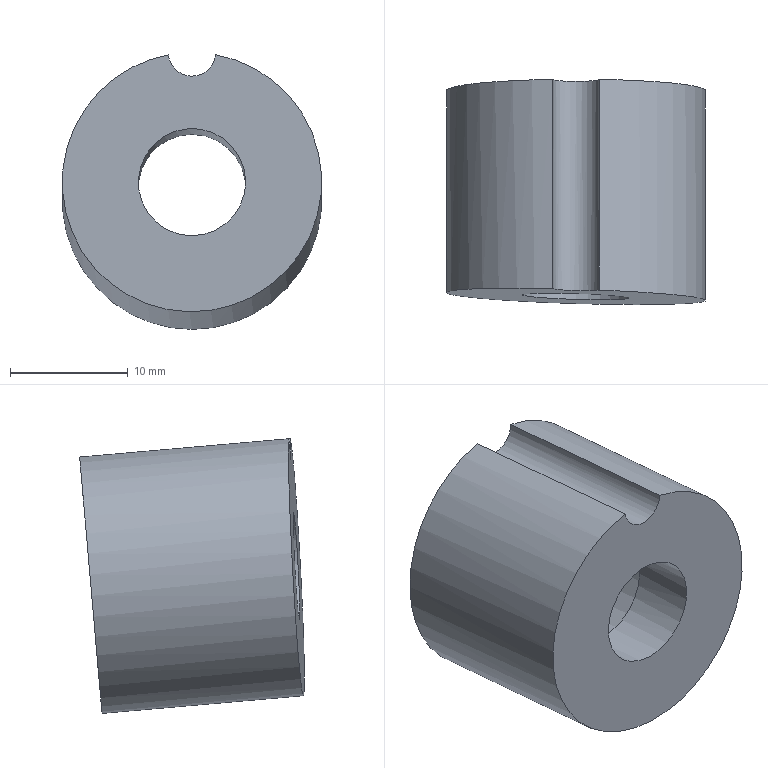Part | NX | features EKSD 22-20-9.100 2 | 1 solid | 7 faces | box 22 x 19.063 x 23.298 mm | volume 4181 mm3 | cylinder 4 | plane 3 | commonest cylinder face diameters 4 x1 9.1 x1 14.6 x1 22 x1
STEP:
#1=CARTESIAN_POINT('',(278.784,-41.385,-40.462));
#2=VERTEX_POINT('',#1);
#3=CARTESIAN_POINT('',(282.767,-41.385,-40.462));
#4=VERTEX_POINT('',#3);
#5=CARTESIAN_POINT('',(280.775,-41.37,-40.281));
#6=DIRECTION('',(0.,-0.9962,0.08716));
#7=DIRECTION('',(0.,-0.08716,-0.9962));
#8=AXIS2_PLACEMENT_3D('',#5,#6,#7);
#9=CIRCLE('',#8,2.);
#10=EDGE_CURVE('',#2,#4,#9,.T.);
#11=ORIENTED_EDGE('',*,*,#10,.T.);
#12=CARTESIAN_POINT('',(280.775,-42.328,-51.239));
#13=DIRECTION('',(0.,-0.9962,0.08716));
#14=DIRECTION('',(0.,-0.08716,-0.9962));
#15=AXIS2_PLACEMENT_3D('',#12,#13,#14);
#16=CIRCLE('',#15,11.);
#17=EDGE_CURVE('',#2,#4,#16,.T.);
#18=ORIENTED_EDGE('',*,*,#17,.F.);
#19=EDGE_LOOP('',(#11,#18));
#20=FACE_BOUND('',#19,.T.);
#21=CARTESIAN_POINT('',(280.775,-41.692,-43.967));
#22=VERTEX_POINT('',#21);
#23=CARTESIAN_POINT('',(280.775,-42.328,-51.239));
#24=DIRECTION('',(0.,0.9962,-0.08716));
#25=DIRECTION('',(0.,0.08716,0.9962));
#26=AXIS2_PLACEMENT_3D('',#23,#24,#25);
#27=CIRCLE('',#26,7.3);
#28=EDGE_CURVE('',#22,#22,#27,.T.);
#29=ORIENTED_EDGE('',*,*,#28,.F.);
#30=EDGE_LOOP('',(#29));
#31=FACE_BOUND('',#30,.T.);
#32=CARTESIAN_POINT('',(280.775,-42.328,-51.239));
#33=DIRECTION('',(0.,0.9962,-0.08716));
#34=DIRECTION('',(0.,0.08716,0.9962));
#35=AXIS2_PLACEMENT_3D('',#32,#33,#34);
#36=PLANE('',#35);
#37=ADVANCED_FACE('',(#20,#31),#36,.T.);
#38=CARTESIAN_POINT('',(282.767,-59.254,-38.899));
#39=VERTEX_POINT('',#38);
#40=CARTESIAN_POINT('',(278.784,-59.133,-38.91));
#41=VERTEX_POINT('',#40);
#42=CARTESIAN_POINT('',(280.775,-59.184,-38.723));
#43=DIRECTION('',(0.03046,0.9981,-0.05344));
#44=DIRECTION('',(-0.6692,-0.01935,-0.7428));
#45=AXIS2_PLACEMENT_3D('',#42,#43,#44);
#46=ELLIPSE('',#45,2.002,2.);
#47=EDGE_CURVE('',#39,#41,#46,.T.);
#48=ORIENTED_EDGE('',*,*,#47,.T.);
#49=CARTESIAN_POINT('',(280.775,-59.772,-49.713));
#50=DIRECTION('',(0.03046,0.9981,-0.05344));
#51=DIRECTION('',(-0.6692,-0.01935,-0.7428));
#52=AXIS2_PLACEMENT_3D('',#49,#50,#51);
#53=ELLIPSE('',#52,11.011,11.);
#54=EDGE_CURVE('',#39,#41,#53,.T.);
#55=ORIENTED_EDGE('',*,*,#54,.F.);
#56=EDGE_LOOP('',(#48,#55));
#57=FACE_BOUND('',#56,.T.);
#58=CARTESIAN_POINT('',(277.727,-59.86,-53.097));
#59=VERTEX_POINT('',#58);
#60=CARTESIAN_POINT('',(280.775,-59.772,-49.713));
#61=DIRECTION('',(0.03046,0.9981,-0.05344));
#62=DIRECTION('',(-0.6692,-0.01935,-0.7428));
#63=AXIS2_PLACEMENT_3D('',#60,#61,#62);
#64=ELLIPSE('',#63,4.555,4.55);
#65=EDGE_CURVE('',#59,#59,#64,.F.);
#66=ORIENTED_EDGE('',*,*,#65,.F.);
#67=EDGE_LOOP('',(#66));
#68=FACE_BOUND('',#67,.T.);
#69=CARTESIAN_POINT('',(457.994,-68.531,-112.302));
#70=DIRECTION('',(0.03046,0.9981,-0.05344));
#71=DIRECTION('',(0.06614,0.05134,0.9965));
#72=AXIS2_PLACEMENT_3D('',#69,#70,#71);
#73=PLANE('',#72);
#74=ADVANCED_FACE('',(#57,#68),#73,.F.);
#75=CARTESIAN_POINT('',(282.767,-51.347,-39.591));
#76=DIRECTION('',(0.,0.9962,-0.08716));
#77=VECTOR('',#76,1000.);
#78=LINE('',#75,#77);
#79=EDGE_CURVE('',#39,#4,#78,.T.);
#80=ORIENTED_EDGE('',*,*,#79,.F.);
#81=ORIENTED_EDGE('',*,*,#54,.T.);
#82=CARTESIAN_POINT('',(278.784,-51.347,-39.591));
#83=DIRECTION('',(0.,0.9962,-0.08716));
#84=VECTOR('',#83,1000.);
#85=LINE('',#82,#84);
#86=EDGE_CURVE('',#2,#41,#85,.F.);
#87=ORIENTED_EDGE('',*,*,#86,.F.);
#88=ORIENTED_EDGE('',*,*,#17,.T.);
#89=EDGE_LOOP('',(#80,#81,#87,#88));
#90=FACE_BOUND('',#89,.T.);
#91=CARTESIAN_POINT('',(280.775,-62.252,-49.496));
#92=DIRECTION('',(0.,0.9962,-0.08716));
#93=DIRECTION('',(0.,0.08716,0.9962));
#94=AXIS2_PLACEMENT_3D('',#91,#92,#93);
#95=CYLINDRICAL_SURFACE('',#94,11.);
#96=ADVANCED_FACE('',(#90),#95,.T.);
#97=CARTESIAN_POINT('',(280.775,-54.679,-54.726));
#98=VERTEX_POINT('',#97);
#99=CARTESIAN_POINT('',(280.775,-54.283,-50.194));
#100=DIRECTION('',(0.,-0.9962,0.08716));
#101=DIRECTION('',(0.,-0.08716,-0.9962));
#102=AXIS2_PLACEMENT_3D('',#99,#100,#101);
#103=CIRCLE('',#102,4.55);
#104=EDGE_CURVE('',#98,#98,#103,.F.);
#105=ORIENTED_EDGE('',*,*,#104,.T.);
#106=EDGE_LOOP('',(#105));
#107=FACE_BOUND('',#106,.T.);
#108=ORIENTED_EDGE('',*,*,#65,.T.);
#109=EDGE_LOOP('',(#108));
#110=FACE_BOUND('',#109,.T.);
#111=CARTESIAN_POINT('',(280.775,-63.248,-49.409));
#112=DIRECTION('',(0.,0.9962,-0.08716));
#113=DIRECTION('',(0.,0.08716,0.9962));
#114=AXIS2_PLACEMENT_3D('',#111,#112,#113);
#115=CYLINDRICAL_SURFACE('',#114,4.55);
#116=ADVANCED_FACE('',(#107,#110),#115,.F.);
#117=CARTESIAN_POINT('',(280.775,-53.646,-42.921));
#118=VERTEX_POINT('',#117);
#119=CARTESIAN_POINT('',(280.775,-54.283,-50.194));
#120=DIRECTION('',(0.,0.9962,-0.08716));
#121=DIRECTION('',(0.,0.08716,0.9962));
#122=AXIS2_PLACEMENT_3D('',#119,#120,#121);
#123=CIRCLE('',#122,7.3);
#124=EDGE_CURVE('',#118,#118,#123,.T.);
#125=ORIENTED_EDGE('',*,*,#124,.T.);
#126=EDGE_LOOP('',(#125));
#127=FACE_BOUND('',#126,.T.);
#128=ORIENTED_EDGE('',*,*,#104,.F.);
#129=EDGE_LOOP('',(#128));
#130=FACE_BOUND('',#129,.T.);
#131=CARTESIAN_POINT('',(280.775,-54.283,-50.194));
#132=DIRECTION('',(0.,-0.9962,0.08716));
#133=DIRECTION('',(0.,-0.08716,-0.9962));
#134=AXIS2_PLACEMENT_3D('',#131,#132,#133);
#135=PLANE('',#134);
#136=ADVANCED_FACE('',(#127,#130),#135,.F.);
#137=ORIENTED_EDGE('',*,*,#28,.T.);
#138=EDGE_LOOP('',(#137));
#139=FACE_BOUND('',#138,.T.);
#140=ORIENTED_EDGE('',*,*,#124,.F.);
#141=EDGE_LOOP('',(#140));
#142=FACE_BOUND('',#141,.T.);
#143=CARTESIAN_POINT('',(280.775,-54.283,-50.194));
#144=DIRECTION('',(0.,0.9962,-0.08716));
#145=DIRECTION('',(0.,0.08716,0.9962));
#146=AXIS2_PLACEMENT_3D('',#143,#144,#145);
#147=CYLINDRICAL_SURFACE('',#146,7.3);
#148=ADVANCED_FACE('',(#139,#142),#147,.F.);
#149=ORIENTED_EDGE('',*,*,#79,.T.);
#150=ORIENTED_EDGE('',*,*,#10,.F.);
#151=ORIENTED_EDGE('',*,*,#86,.T.);
#152=ORIENTED_EDGE('',*,*,#47,.F.);
#153=EDGE_LOOP('',(#149,#150,#151,#152));
#154=FACE_BOUND('',#153,.T.);
#155=CARTESIAN_POINT('',(280.775,-61.294,-38.538));
#156=DIRECTION('',(0.,0.9962,-0.08716));
#157=DIRECTION('',(0.,0.08716,0.9962));
#158=AXIS2_PLACEMENT_3D('',#155,#156,#157);
#159=CYLINDRICAL_SURFACE('',#158,2.);
#160=ADVANCED_FACE('',(#154),#159,.F.);
#161=CLOSED_SHELL('',(#37,#74,#96,#116,#136,#148,#160));
#162=MANIFOLD_SOLID_BREP('',#161);
#163=(LENGTH_UNIT()NAMED_UNIT(*)SI_UNIT(.MILLI.,.METRE.));
#164=UNCERTAINTY_MEASURE_WITH_UNIT(LENGTH_MEASURE(0.00001),#163,'','');
#165=(NAMED_UNIT(*)PLANE_ANGLE_UNIT()SI_UNIT($,.RADIAN.));
#166=(NAMED_UNIT(*)SI_UNIT($,.STERADIAN.)SOLID_ANGLE_UNIT());
#167=(GEOMETRIC_REPRESENTATION_CONTEXT(3)GLOBAL_UNCERTAINTY_ASSIGNED_CONTEXT((#164))GLOBAL_UNIT_ASSIGNED_CONTEXT((#163,#165,#166))REPRESENTATION_CONTEXT('',''));
#168=ADVANCED_BREP_SHAPE_REPRESENTATION('',(#162),#167);